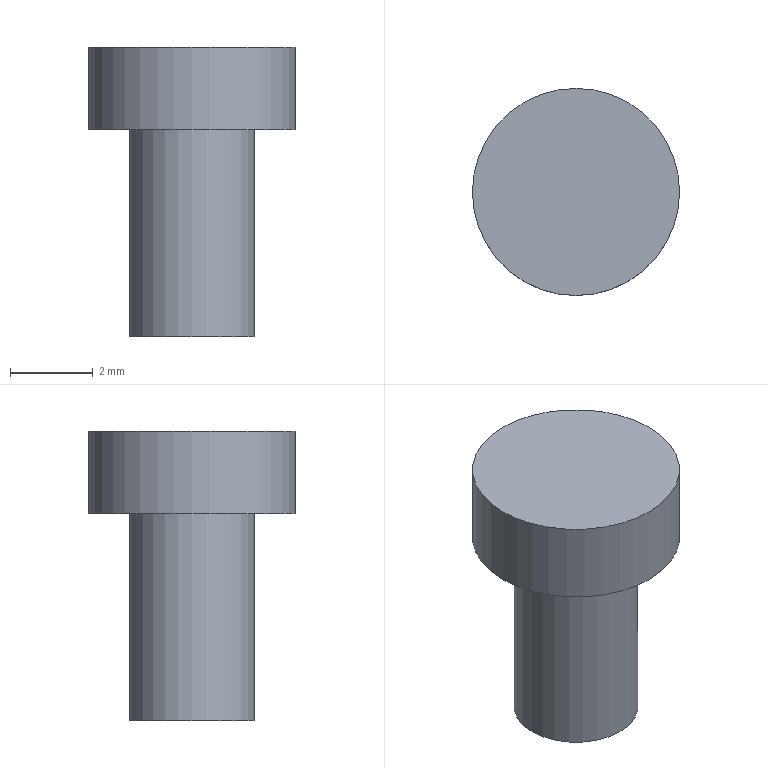Part | NX | features CYLINDER 2, DATUM_CSYS 1 | 1 solid | 5 faces | box 5 x 5 x 7 mm | volume 74.613 mm3 | plane 3 | cylinder 2 | commonest cylinder face diameters 3 x1 5 x1
STEP:
#1=CARTESIAN_POINT('',(1.5,0.,0.));
#2=VERTEX_POINT('',#1);
#3=CARTESIAN_POINT('',(0.,0.,0.));
#4=DIRECTION('',(0.,0.,1.));
#5=DIRECTION('',(1.,0.,0.));
#6=AXIS2_PLACEMENT_3D('',#3,#4,#5);
#7=CIRCLE('',#6,1.5);
#8=EDGE_CURVE('',#2,#2,#7,.T.);
#9=ORIENTED_EDGE('',*,*,#8,.F.);
#10=EDGE_LOOP('',(#9));
#11=FACE_BOUND('',#10,.T.);
#12=CARTESIAN_POINT('',(0.,0.,0.));
#13=DIRECTION('',(0.,0.,-1.));
#14=DIRECTION('',(-1.,0.,0.));
#15=AXIS2_PLACEMENT_3D('',#12,#13,#14);
#16=PLANE('',#15);
#17=ADVANCED_FACE('',(#11),#16,.T.);
#18=CARTESIAN_POINT('',(1.5,0.,5.));
#19=VERTEX_POINT('',#18);
#20=CARTESIAN_POINT('',(0.,0.,5.));
#21=DIRECTION('',(0.,0.,-1.));
#22=DIRECTION('',(1.,0.,0.));
#23=AXIS2_PLACEMENT_3D('',#20,#21,#22);
#24=CIRCLE('',#23,1.5);
#25=EDGE_CURVE('',#19,#19,#24,.T.);
#26=ORIENTED_EDGE('',*,*,#25,.T.);
#27=EDGE_LOOP('',(#26));
#28=FACE_BOUND('',#27,.T.);
#29=ORIENTED_EDGE('',*,*,#8,.T.);
#30=EDGE_LOOP('',(#29));
#31=FACE_BOUND('',#30,.T.);
#32=CARTESIAN_POINT('',(0.,0.,0.));
#33=DIRECTION('',(0.,0.,1.));
#34=DIRECTION('',(1.,0.,0.));
#35=AXIS2_PLACEMENT_3D('',#32,#33,#34);
#36=CYLINDRICAL_SURFACE('',#35,1.5);
#37=ADVANCED_FACE('',(#28,#31),#36,.T.);
#38=CARTESIAN_POINT('',(2.5,0.,7.));
#39=VERTEX_POINT('',#38);
#40=CARTESIAN_POINT('',(0.,0.,7.));
#41=DIRECTION('',(0.,0.,-1.));
#42=DIRECTION('',(1.,0.,0.));
#43=AXIS2_PLACEMENT_3D('',#40,#41,#42);
#44=CIRCLE('',#43,2.5);
#45=EDGE_CURVE('',#39,#39,#44,.T.);
#46=ORIENTED_EDGE('',*,*,#45,.F.);
#47=EDGE_LOOP('',(#46));
#48=FACE_BOUND('',#47,.T.);
#49=CARTESIAN_POINT('',(0.,0.,7.));
#50=DIRECTION('',(0.,0.,1.));
#51=DIRECTION('',(1.,0.,0.));
#52=AXIS2_PLACEMENT_3D('',#49,#50,#51);
#53=PLANE('',#52);
#54=ADVANCED_FACE('',(#48),#53,.T.);
#55=ORIENTED_EDGE('',*,*,#25,.F.);
#56=EDGE_LOOP('',(#55));
#57=FACE_BOUND('',#56,.T.);
#58=CARTESIAN_POINT('',(2.5,0.,5.));
#59=VERTEX_POINT('',#58);
#60=CARTESIAN_POINT('',(0.,0.,5.));
#61=DIRECTION('',(0.,0.,1.));
#62=DIRECTION('',(1.,0.,0.));
#63=AXIS2_PLACEMENT_3D('',#60,#61,#62);
#64=CIRCLE('',#63,2.5);
#65=EDGE_CURVE('',#59,#59,#64,.T.);
#66=ORIENTED_EDGE('',*,*,#65,.F.);
#67=EDGE_LOOP('',(#66));
#68=FACE_BOUND('',#67,.T.);
#69=CARTESIAN_POINT('',(0.,0.,5.));
#70=DIRECTION('',(0.,0.,-1.));
#71=DIRECTION('',(-1.,0.,0.));
#72=AXIS2_PLACEMENT_3D('',#69,#70,#71);
#73=PLANE('',#72);
#74=ADVANCED_FACE('',(#57,#68),#73,.T.);
#75=ORIENTED_EDGE('',*,*,#45,.T.);
#76=EDGE_LOOP('',(#75));
#77=FACE_BOUND('',#76,.T.);
#78=ORIENTED_EDGE('',*,*,#65,.T.);
#79=EDGE_LOOP('',(#78));
#80=FACE_BOUND('',#79,.T.);
#81=CARTESIAN_POINT('',(0.,0.,5.));
#82=DIRECTION('',(0.,0.,1.));
#83=DIRECTION('',(1.,0.,0.));
#84=AXIS2_PLACEMENT_3D('',#81,#82,#83);
#85=CYLINDRICAL_SURFACE('',#84,2.5);
#86=ADVANCED_FACE('',(#77,#80),#85,.T.);
#87=CLOSED_SHELL('',(#17,#37,#54,#74,#86));
#88=MANIFOLD_SOLID_BREP('',#87);
#89=(LENGTH_UNIT()NAMED_UNIT(*)SI_UNIT(.MILLI.,.METRE.));
#90=UNCERTAINTY_MEASURE_WITH_UNIT(LENGTH_MEASURE(0.00001),#89,'','');
#91=(NAMED_UNIT(*)PLANE_ANGLE_UNIT()SI_UNIT($,.RADIAN.));
#92=(NAMED_UNIT(*)SI_UNIT($,.STERADIAN.)SOLID_ANGLE_UNIT());
#93=(GEOMETRIC_REPRESENTATION_CONTEXT(3)GLOBAL_UNCERTAINTY_ASSIGNED_CONTEXT((#90))GLOBAL_UNIT_ASSIGNED_CONTEXT((#89,#91,#92))REPRESENTATION_CONTEXT('',''));
#94=ADVANCED_BREP_SHAPE_REPRESENTATION('',(#88),#93);